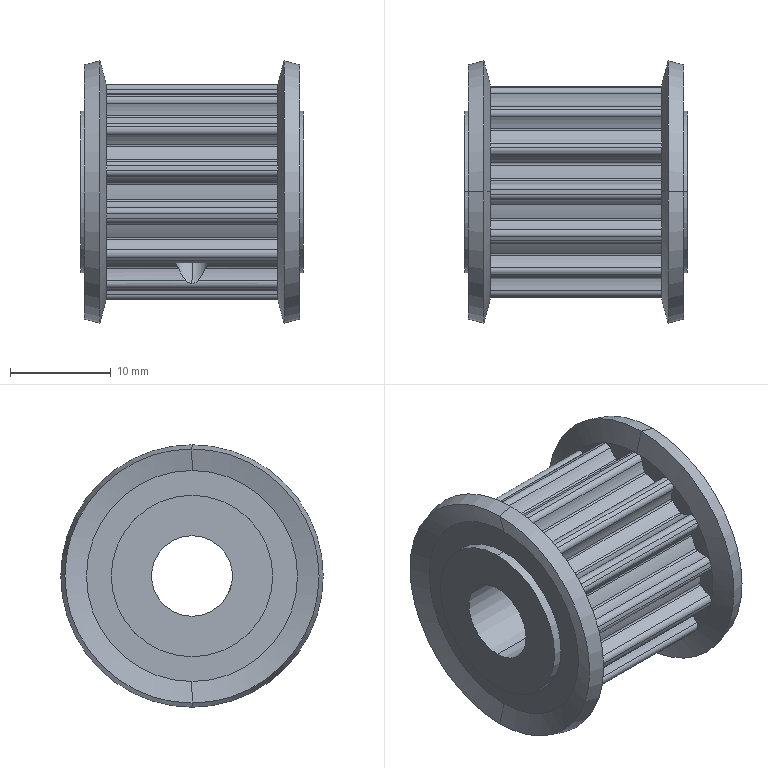Part | SolidWorks | 3 solids | 221 faces | box 22 x 26 x 26 mm | volume 5822 mm3 | cylinder 137 | plane 60 | cone 24 | commonest cylinder face diameters 0.5 x32 6.55 x32 1.1 x28 17.78 x16 21.32 x15 3.242 x4